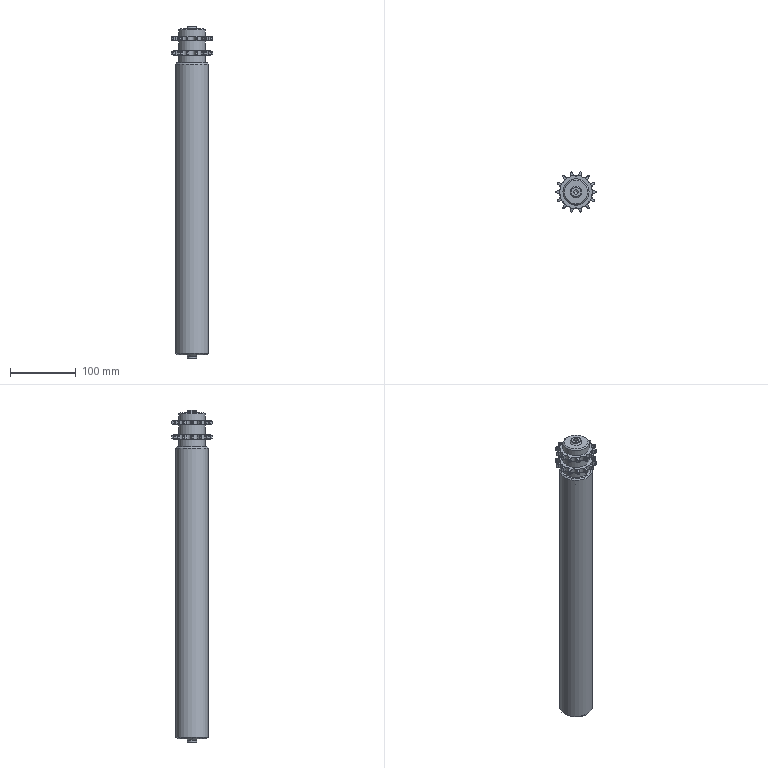Part | STEP file | 08b1-14 | 2 solids | 308 faces | box 63.262 x 61.879 x 506 mm | volume 1624253 mm3 | cylinder 176 | plane 67 | torus 56 | cone 5 | spline 4 | commonest cylinder face diameters 14.27 x56 22.211 x56 8.595 x28 63.262 x28 14 x3 40 x3